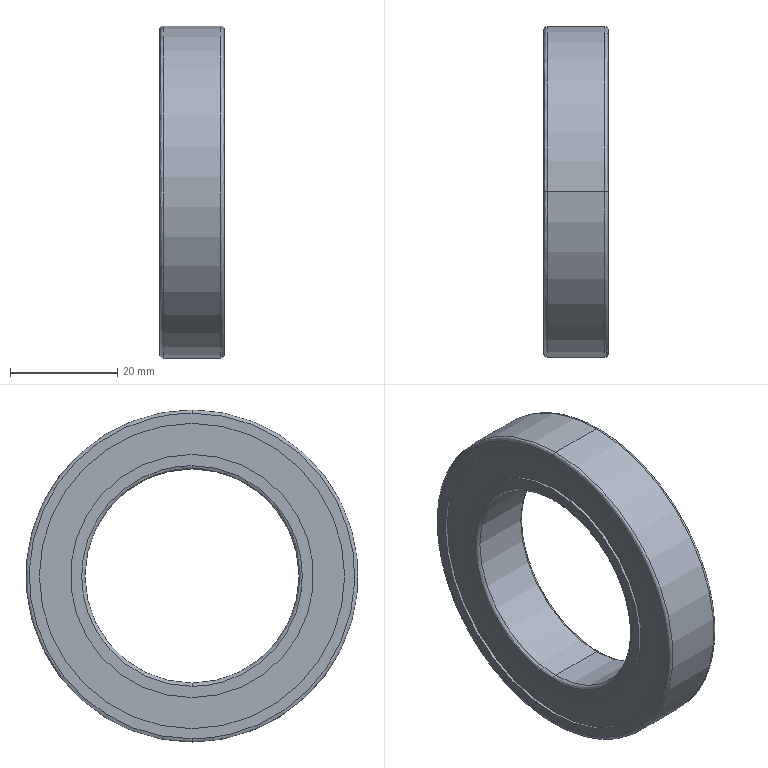Part | STEP file | B6908ZZ_Default | 1 solid | 26 faces | box 12 x 62 x 62 mm | volume 20172 mm3 | cylinder 12 | spline 8 | plane 6 | commonest cylinder face diameters 45.4 x4 57 x4 40 x2 62 x2